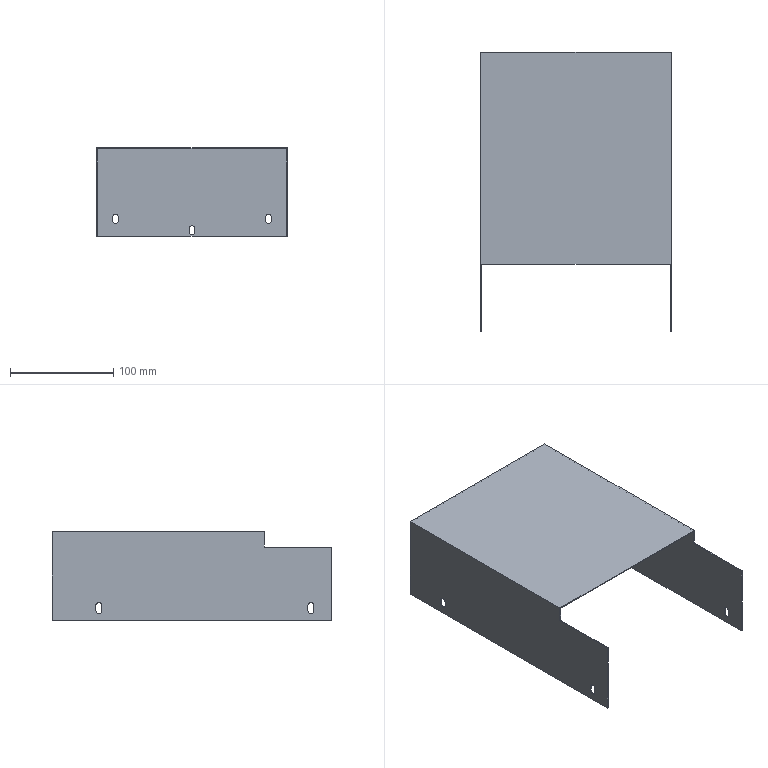Part | SolidWorks | features HoleWzd 2, Extrusion 1, ICE 1, Shell 1 | 1 solid | 49 faces | box 184 x 270 x 86 mm | volume 96917 mm3 | plane 28 | cylinder 21 | commonest cylinder face diameters 5.8 x21